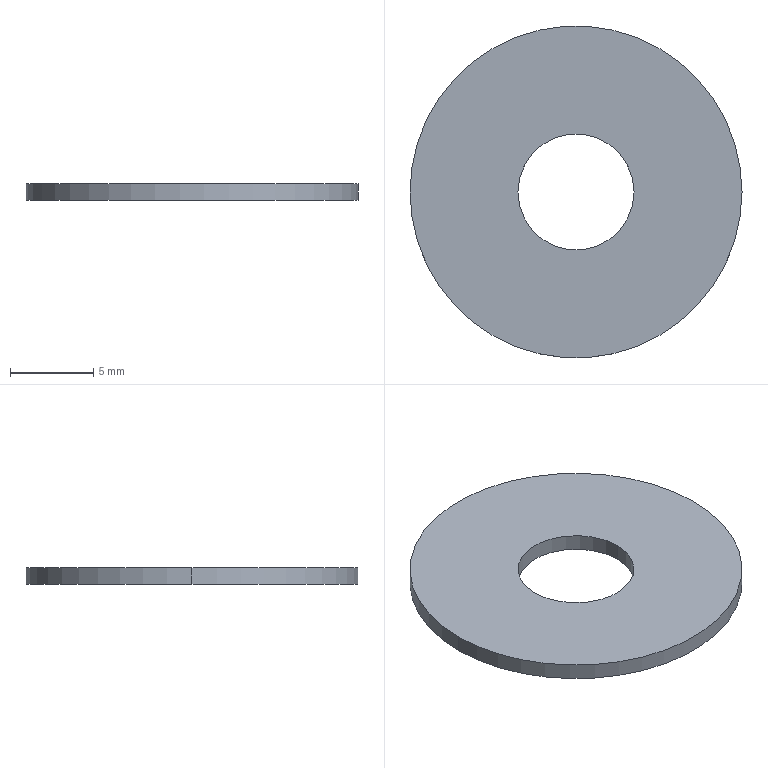Part | SolidWorks | features Extrusion 1 | 1 solid | 6 faces | box 20 x 20 x 1 mm | volume 275.675 mm3 | cylinder 4 | plane 2 | commonest cylinder face diameters 7 x2 20 x2
STEP:
#1=CARTESIAN_POINT('',(-3.5,0.,1.));
#2=VERTEX_POINT('',#1);
#3=CARTESIAN_POINT('',(3.5,0.,1.));
#4=VERTEX_POINT('',#3);
#5=CARTESIAN_POINT('',(0.,0.,1.));
#6=DIRECTION('',(0.,0.,1.));
#7=DIRECTION('',(1.,0.,0.));
#8=AXIS2_PLACEMENT_3D('',#5,#6,#7);
#9=CIRCLE('',#8,3.5);
#10=EDGE_CURVE('',#2,#4,#9,.T.);
#11=ORIENTED_EDGE('',*,*,#10,.T.);
#12=CARTESIAN_POINT('',(3.5,0.,0.));
#13=VERTEX_POINT('',#12);
#14=CARTESIAN_POINT('',(3.5,0.,1.));
#15=DIRECTION('',(0.,0.,-1.));
#16=VECTOR('',#15,1000.);
#17=LINE('',#14,#16);
#18=EDGE_CURVE('',#4,#13,#17,.T.);
#19=ORIENTED_EDGE('',*,*,#18,.T.);
#20=CARTESIAN_POINT('',(-3.5,0.,0.));
#21=VERTEX_POINT('',#20);
#22=CARTESIAN_POINT('',(0.,0.,0.));
#23=DIRECTION('',(0.,0.,1.));
#24=DIRECTION('',(1.,0.,0.));
#25=AXIS2_PLACEMENT_3D('',#22,#23,#24);
#26=CIRCLE('',#25,3.5);
#27=EDGE_CURVE('',#21,#13,#26,.T.);
#28=ORIENTED_EDGE('',*,*,#27,.F.);
#29=CARTESIAN_POINT('',(-3.5,0.,1.));
#30=DIRECTION('',(0.,0.,-1.));
#31=VECTOR('',#30,1000.);
#32=LINE('',#29,#31);
#33=EDGE_CURVE('',#2,#21,#32,.T.);
#34=ORIENTED_EDGE('',*,*,#33,.F.);
#35=EDGE_LOOP('',(#11,#19,#28,#34));
#36=FACE_OUTER_BOUND('',#35,.T.);
#37=CARTESIAN_POINT('',(0.,0.,1.));
#38=DIRECTION('',(0.,0.,-1.));
#39=DIRECTION('',(-1.,0.,0.));
#40=AXIS2_PLACEMENT_3D('',#37,#38,#39);
#41=CYLINDRICAL_SURFACE('',#40,3.5);
#42=ADVANCED_FACE('',(#36),#41,.F.);
#43=CARTESIAN_POINT('',(10.,0.,1.));
#44=VERTEX_POINT('',#43);
#45=CARTESIAN_POINT('',(-10.,0.,1.));
#46=VERTEX_POINT('',#45);
#47=CARTESIAN_POINT('',(0.,0.,1.));
#48=DIRECTION('',(0.,0.,1.));
#49=DIRECTION('',(1.,0.,0.));
#50=AXIS2_PLACEMENT_3D('',#47,#48,#49);
#51=CIRCLE('',#50,10.);
#52=EDGE_CURVE('',#44,#46,#51,.T.);
#53=ORIENTED_EDGE('',*,*,#52,.F.);
#54=CARTESIAN_POINT('',(10.,0.,0.));
#55=VERTEX_POINT('',#54);
#56=CARTESIAN_POINT('',(10.,0.,1.));
#57=DIRECTION('',(0.,0.,-1.));
#58=VECTOR('',#57,1000.);
#59=LINE('',#56,#58);
#60=EDGE_CURVE('',#44,#55,#59,.T.);
#61=ORIENTED_EDGE('',*,*,#60,.T.);
#62=CARTESIAN_POINT('',(-10.,0.,0.));
#63=VERTEX_POINT('',#62);
#64=CARTESIAN_POINT('',(0.,0.,0.));
#65=DIRECTION('',(0.,0.,1.));
#66=DIRECTION('',(1.,0.,0.));
#67=AXIS2_PLACEMENT_3D('',#64,#65,#66);
#68=CIRCLE('',#67,10.);
#69=EDGE_CURVE('',#55,#63,#68,.T.);
#70=ORIENTED_EDGE('',*,*,#69,.T.);
#71=CARTESIAN_POINT('',(-10.,0.,1.));
#72=DIRECTION('',(0.,0.,-1.));
#73=VECTOR('',#72,1000.);
#74=LINE('',#71,#73);
#75=EDGE_CURVE('',#46,#63,#74,.T.);
#76=ORIENTED_EDGE('',*,*,#75,.F.);
#77=EDGE_LOOP('',(#53,#61,#70,#76));
#78=FACE_OUTER_BOUND('',#77,.T.);
#79=CARTESIAN_POINT('',(0.,0.,1.));
#80=DIRECTION('',(0.,0.,-1.));
#81=DIRECTION('',(-1.,0.,0.));
#82=AXIS2_PLACEMENT_3D('',#79,#80,#81);
#83=CYLINDRICAL_SURFACE('',#82,10.);
#84=ADVANCED_FACE('',(#78),#83,.T.);
#85=CARTESIAN_POINT('',(0.,0.,1.));
#86=DIRECTION('',(0.,0.,1.));
#87=DIRECTION('',(1.,0.,0.));
#88=AXIS2_PLACEMENT_3D('',#85,#86,#87);
#89=CIRCLE('',#88,10.);
#90=EDGE_CURVE('',#46,#44,#89,.T.);
#91=ORIENTED_EDGE('',*,*,#90,.T.);
#92=ORIENTED_EDGE('',*,*,#52,.T.);
#93=EDGE_LOOP('',(#91,#92));
#94=FACE_OUTER_BOUND('',#93,.T.);
#95=ORIENTED_EDGE('',*,*,#10,.F.);
#96=CARTESIAN_POINT('',(0.,0.,1.));
#97=DIRECTION('',(0.,0.,1.));
#98=DIRECTION('',(1.,0.,0.));
#99=AXIS2_PLACEMENT_3D('',#96,#97,#98);
#100=CIRCLE('',#99,3.5);
#101=EDGE_CURVE('',#4,#2,#100,.T.);
#102=ORIENTED_EDGE('',*,*,#101,.F.);
#103=EDGE_LOOP('',(#95,#102));
#104=FACE_BOUND('',#103,.T.);
#105=CARTESIAN_POINT('',(0.,0.,1.));
#106=DIRECTION('',(0.,0.,1.));
#107=DIRECTION('',(1.,0.,0.));
#108=AXIS2_PLACEMENT_3D('',#105,#106,#107);
#109=PLANE('',#108);
#110=ADVANCED_FACE('',(#94,#104),#109,.T.);
#111=CARTESIAN_POINT('',(0.,0.,0.));
#112=DIRECTION('',(0.,0.,1.));
#113=DIRECTION('',(1.,0.,0.));
#114=AXIS2_PLACEMENT_3D('',#111,#112,#113);
#115=CIRCLE('',#114,10.);
#116=EDGE_CURVE('',#63,#55,#115,.T.);
#117=ORIENTED_EDGE('',*,*,#116,.F.);
#118=ORIENTED_EDGE('',*,*,#69,.F.);
#119=EDGE_LOOP('',(#117,#118));
#120=FACE_OUTER_BOUND('',#119,.T.);
#121=ORIENTED_EDGE('',*,*,#27,.T.);
#122=CARTESIAN_POINT('',(0.,0.,0.));
#123=DIRECTION('',(0.,0.,1.));
#124=DIRECTION('',(1.,0.,0.));
#125=AXIS2_PLACEMENT_3D('',#122,#123,#124);
#126=CIRCLE('',#125,3.5);
#127=EDGE_CURVE('',#13,#21,#126,.T.);
#128=ORIENTED_EDGE('',*,*,#127,.T.);
#129=EDGE_LOOP('',(#121,#128));
#130=FACE_BOUND('',#129,.T.);
#131=CARTESIAN_POINT('',(0.,0.,0.));
#132=DIRECTION('',(0.,0.,1.));
#133=DIRECTION('',(1.,0.,0.));
#134=AXIS2_PLACEMENT_3D('',#131,#132,#133);
#135=PLANE('',#134);
#136=ADVANCED_FACE('',(#120,#130),#135,.F.);
#137=ORIENTED_EDGE('',*,*,#60,.F.);
#138=ORIENTED_EDGE('',*,*,#90,.F.);
#139=ORIENTED_EDGE('',*,*,#75,.T.);
#140=ORIENTED_EDGE('',*,*,#116,.T.);
#141=EDGE_LOOP('',(#137,#138,#139,#140));
#142=FACE_OUTER_BOUND('',#141,.T.);
#143=CARTESIAN_POINT('',(0.,0.,1.));
#144=DIRECTION('',(0.,0.,-1.));
#145=DIRECTION('',(-1.,0.,0.));
#146=AXIS2_PLACEMENT_3D('',#143,#144,#145);
#147=CYLINDRICAL_SURFACE('',#146,10.);
#148=ADVANCED_FACE('',(#142),#147,.T.);
#149=ORIENTED_EDGE('',*,*,#18,.F.);
#150=ORIENTED_EDGE('',*,*,#101,.T.);
#151=ORIENTED_EDGE('',*,*,#33,.T.);
#152=ORIENTED_EDGE('',*,*,#127,.F.);
#153=EDGE_LOOP('',(#149,#150,#151,#152));
#154=FACE_OUTER_BOUND('',#153,.T.);
#155=CARTESIAN_POINT('',(0.,0.,1.));
#156=DIRECTION('',(0.,0.,-1.));
#157=DIRECTION('',(-1.,0.,0.));
#158=AXIS2_PLACEMENT_3D('',#155,#156,#157);
#159=CYLINDRICAL_SURFACE('',#158,3.5);
#160=ADVANCED_FACE('',(#154),#159,.F.);
#161=CLOSED_SHELL('',(#42,#84,#110,#136,#148,#160));
#162=MANIFOLD_SOLID_BREP('',#161);
#163=CARTESIAN_POINT('',(0.,0.,0.));
#164=DIRECTION('',(0.,0.,1.));
#165=DIRECTION('',(1.,0.,0.));
#166=AXIS2_PLACEMENT_3D('',#163,#164,#165);
#167=(LENGTH_UNIT()NAMED_UNIT(*)SI_UNIT(.MILLI.,.METRE.));
#168=UNCERTAINTY_MEASURE_WITH_UNIT(LENGTH_MEASURE(0.00001),#167,'','');
#169=(NAMED_UNIT(*)PLANE_ANGLE_UNIT()SI_UNIT($,.RADIAN.));
#170=(NAMED_UNIT(*)SI_UNIT($,.STERADIAN.)SOLID_ANGLE_UNIT());
#171=(GEOMETRIC_REPRESENTATION_CONTEXT(3)GLOBAL_UNCERTAINTY_ASSIGNED_CONTEXT((#168))GLOBAL_UNIT_ASSIGNED_CONTEXT((#167,#169,#170))REPRESENTATION_CONTEXT('',''));
#172=ADVANCED_BREP_SHAPE_REPRESENTATION('',(#162,#166),#171);